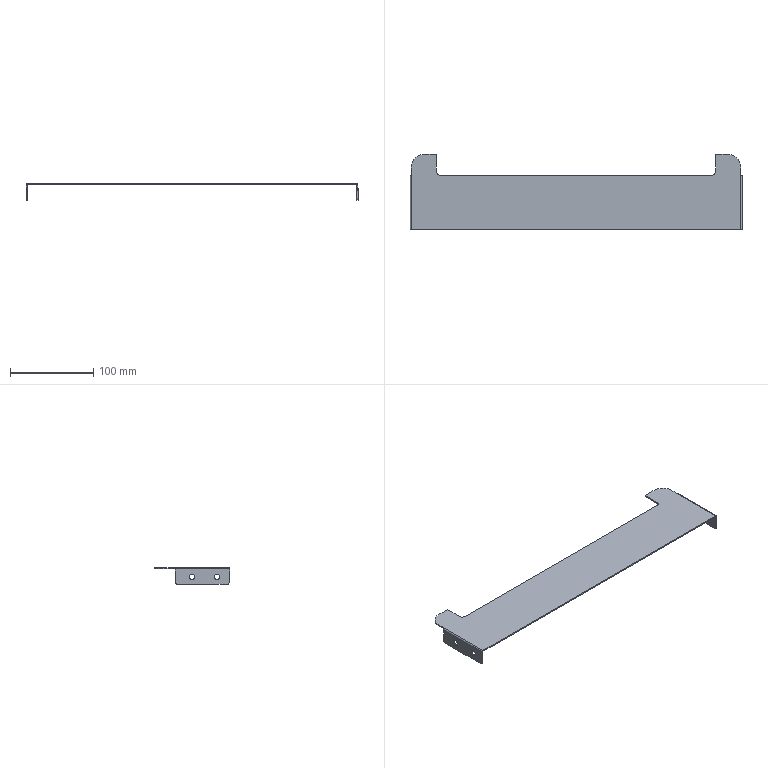Part | SolidWorks | features Fillet 3, EdgeFlange 1, FlatPattern 1, HoleWzd 1, ICE 1, SMBaseFlange 1, SheetMetal 1 | 1 solid | 42 faces | box 398 x 90 x 20 mm | volume 44260 mm3 | plane 24 | cylinder 18 | commonest cylinder face diameters 6.5 x8 6 x4 3 x2 10 x2 30 x2
STEP:
#1=CARTESIAN_POINT('',(199.,0.,-14.25));
#2=VERTEX_POINT('',#1);
#3=CARTESIAN_POINT('',(199.,0.,-7.75));
#4=VERTEX_POINT('',#3);
#5=CARTESIAN_POINT('',(199.,0.,-11.));
#6=DIRECTION('',(-1.,0.,0.));
#7=DIRECTION('',(0.,0.,1.));
#8=AXIS2_PLACEMENT_3D('',#5,#6,#7);
#9=CIRCLE('',#8,3.25);
#10=EDGE_CURVE('',#2,#4,#9,.T.);
#11=ORIENTED_EDGE('',*,*,#10,.F.);
#12=CARTESIAN_POINT('',(197.5,0.,-14.25));
#13=VERTEX_POINT('',#12);
#14=CARTESIAN_POINT('',(-199.,0.,-14.25));
#15=DIRECTION('',(-1.,0.,0.));
#16=VECTOR('',#15,1000.);
#17=LINE('',#14,#16);
#18=EDGE_CURVE('',#2,#13,#17,.T.);
#19=ORIENTED_EDGE('',*,*,#18,.T.);
#20=CARTESIAN_POINT('',(197.5,0.,-7.75));
#21=VERTEX_POINT('',#20);
#22=CARTESIAN_POINT('',(197.5,0.,-11.));
#23=DIRECTION('',(-1.,0.,0.));
#24=DIRECTION('',(0.,0.,1.));
#25=AXIS2_PLACEMENT_3D('',#22,#23,#24);
#26=CIRCLE('',#25,3.25);
#27=EDGE_CURVE('',#13,#21,#26,.T.);
#28=ORIENTED_EDGE('',*,*,#27,.T.);
#29=CARTESIAN_POINT('',(-199.,0.,-7.75));
#30=DIRECTION('',(-1.,0.,0.));
#31=VECTOR('',#30,1000.);
#32=LINE('',#29,#31);
#33=EDGE_CURVE('',#4,#21,#32,.T.);
#34=ORIENTED_EDGE('',*,*,#33,.F.);
#35=EDGE_LOOP('',(#11,#19,#28,#34));
#36=FACE_OUTER_BOUND('',#35,.T.);
#37=CARTESIAN_POINT('',(-199.,0.,-11.));
#38=DIRECTION('',(-1.,0.,0.));
#39=DIRECTION('',(0.,0.,1.));
#40=AXIS2_PLACEMENT_3D('',#37,#38,#39);
#41=CYLINDRICAL_SURFACE('',#40,3.25);
#42=ADVANCED_FACE('',(#36),#41,.F.);
#43=CARTESIAN_POINT('',(-197.5,0.,-14.25));
#44=VERTEX_POINT('',#43);
#45=CARTESIAN_POINT('',(-197.5,0.,-7.75));
#46=VERTEX_POINT('',#45);
#47=CARTESIAN_POINT('',(-197.5,0.,-11.));
#48=DIRECTION('',(-1.,0.,0.));
#49=DIRECTION('',(0.,0.,1.));
#50=AXIS2_PLACEMENT_3D('',#47,#48,#49);
#51=CIRCLE('',#50,3.25);
#52=EDGE_CURVE('',#44,#46,#51,.T.);
#53=ORIENTED_EDGE('',*,*,#52,.F.);
#54=CARTESIAN_POINT('',(-199.,0.,-14.25));
#55=VERTEX_POINT('',#54);
#56=CARTESIAN_POINT('',(-199.,0.,-14.25));
#57=DIRECTION('',(-1.,0.,0.));
#58=VECTOR('',#57,1000.);
#59=LINE('',#56,#58);
#60=EDGE_CURVE('',#44,#55,#59,.T.);
#61=ORIENTED_EDGE('',*,*,#60,.T.);
#62=CARTESIAN_POINT('',(-199.,0.,-7.75));
#63=VERTEX_POINT('',#62);
#64=CARTESIAN_POINT('',(-199.,0.,-11.));
#65=DIRECTION('',(-1.,0.,0.));
#66=DIRECTION('',(0.,0.,1.));
#67=AXIS2_PLACEMENT_3D('',#64,#65,#66);
#68=CIRCLE('',#67,3.25);
#69=EDGE_CURVE('',#55,#63,#68,.T.);
#70=ORIENTED_EDGE('',*,*,#69,.T.);
#71=CARTESIAN_POINT('',(-199.,0.,-7.75));
#72=DIRECTION('',(-1.,0.,0.));
#73=VECTOR('',#72,1000.);
#74=LINE('',#71,#73);
#75=EDGE_CURVE('',#46,#63,#74,.T.);
#76=ORIENTED_EDGE('',*,*,#75,.F.);
#77=EDGE_LOOP('',(#53,#61,#70,#76));
#78=FACE_OUTER_BOUND('',#77,.T.);
#79=CARTESIAN_POINT('',(-199.,0.,-11.));
#80=DIRECTION('',(-1.,0.,0.));
#81=DIRECTION('',(0.,0.,1.));
#82=AXIS2_PLACEMENT_3D('',#79,#80,#81);
#83=CYLINDRICAL_SURFACE('',#82,3.25);
#84=ADVANCED_FACE('',(#78),#83,.F.);
#85=CARTESIAN_POINT('',(-197.5,-30.,-14.25));
#86=VERTEX_POINT('',#85);
#87=CARTESIAN_POINT('',(-197.5,-30.,-7.75));
#88=VERTEX_POINT('',#87);
#89=CARTESIAN_POINT('',(-197.5,-30.,-11.));
#90=DIRECTION('',(-1.,0.,0.));
#91=DIRECTION('',(0.,0.,1.));
#92=AXIS2_PLACEMENT_3D('',#89,#90,#91);
#93=CIRCLE('',#92,3.25);
#94=EDGE_CURVE('',#86,#88,#93,.T.);
#95=ORIENTED_EDGE('',*,*,#94,.F.);
#96=CARTESIAN_POINT('',(-199.,-30.,-14.25));
#97=VERTEX_POINT('',#96);
#98=CARTESIAN_POINT('',(-199.,-30.,-14.25));
#99=DIRECTION('',(-1.,0.,0.));
#100=VECTOR('',#99,1000.);
#101=LINE('',#98,#100);
#102=EDGE_CURVE('',#86,#97,#101,.T.);
#103=ORIENTED_EDGE('',*,*,#102,.T.);
#104=CARTESIAN_POINT('',(-199.,-30.,-7.75));
#105=VERTEX_POINT('',#104);
#106=CARTESIAN_POINT('',(-199.,-30.,-11.));
#107=DIRECTION('',(-1.,0.,0.));
#108=DIRECTION('',(0.,0.,1.));
#109=AXIS2_PLACEMENT_3D('',#106,#107,#108);
#110=CIRCLE('',#109,3.25);
#111=EDGE_CURVE('',#97,#105,#110,.T.);
#112=ORIENTED_EDGE('',*,*,#111,.T.);
#113=CARTESIAN_POINT('',(-199.,-30.,-7.75));
#114=DIRECTION('',(-1.,0.,0.));
#115=VECTOR('',#114,1000.);
#116=LINE('',#113,#115);
#117=EDGE_CURVE('',#88,#105,#116,.T.);
#118=ORIENTED_EDGE('',*,*,#117,.F.);
#119=EDGE_LOOP('',(#95,#103,#112,#118));
#120=FACE_OUTER_BOUND('',#119,.T.);
#121=CARTESIAN_POINT('',(-199.,-30.,-11.));
#122=DIRECTION('',(-1.,0.,0.));
#123=DIRECTION('',(0.,0.,1.));
#124=AXIS2_PLACEMENT_3D('',#121,#122,#123);
#125=CYLINDRICAL_SURFACE('',#124,3.25);
#126=ADVANCED_FACE('',(#120),#125,.F.);
#127=CARTESIAN_POINT('',(199.,-30.,-14.25));
#128=VERTEX_POINT('',#127);
#129=CARTESIAN_POINT('',(199.,-30.,-7.75));
#130=VERTEX_POINT('',#129);
#131=CARTESIAN_POINT('',(199.,-30.,-11.));
#132=DIRECTION('',(-1.,0.,0.));
#133=DIRECTION('',(0.,0.,1.));
#134=AXIS2_PLACEMENT_3D('',#131,#132,#133);
#135=CIRCLE('',#134,3.25);
#136=EDGE_CURVE('',#128,#130,#135,.T.);
#137=ORIENTED_EDGE('',*,*,#136,.F.);
#138=CARTESIAN_POINT('',(197.5,-30.,-14.25));
#139=VERTEX_POINT('',#138);
#140=CARTESIAN_POINT('',(-199.,-30.,-14.25));
#141=DIRECTION('',(-1.,0.,0.));
#142=VECTOR('',#141,1000.);
#143=LINE('',#140,#142);
#144=EDGE_CURVE('',#128,#139,#143,.T.);
#145=ORIENTED_EDGE('',*,*,#144,.T.);
#146=CARTESIAN_POINT('',(197.5,-30.,-7.75));
#147=VERTEX_POINT('',#146);
#148=CARTESIAN_POINT('',(197.5,-30.,-11.));
#149=DIRECTION('',(-1.,0.,0.));
#150=DIRECTION('',(0.,0.,1.));
#151=AXIS2_PLACEMENT_3D('',#148,#149,#150);
#152=CIRCLE('',#151,3.25);
#153=EDGE_CURVE('',#139,#147,#152,.T.);
#154=ORIENTED_EDGE('',*,*,#153,.T.);
#155=CARTESIAN_POINT('',(-199.,-30.,-7.75));
#156=DIRECTION('',(-1.,0.,0.));
#157=VECTOR('',#156,1000.);
#158=LINE('',#155,#157);
#159=EDGE_CURVE('',#130,#147,#158,.T.);
#160=ORIENTED_EDGE('',*,*,#159,.F.);
#161=EDGE_LOOP('',(#137,#145,#154,#160));
#162=FACE_OUTER_BOUND('',#161,.T.);
#163=CARTESIAN_POINT('',(-199.,-30.,-11.));
#164=DIRECTION('',(-1.,0.,0.));
#165=DIRECTION('',(0.,0.,1.));
#166=AXIS2_PLACEMENT_3D('',#163,#164,#165);
#167=CYLINDRICAL_SURFACE('',#166,3.25);
#168=ADVANCED_FACE('',(#162),#167,.F.);
#169=CARTESIAN_POINT('',(-167.5,45.,-1.5));
#170=VERTEX_POINT('',#169);
#171=CARTESIAN_POINT('',(-167.5,45.,0.));
#172=VERTEX_POINT('',#171);
#173=CARTESIAN_POINT('',(-167.5,45.,-1.5));
#174=DIRECTION('',(0.,0.,1.));
#175=VECTOR('',#174,1000.);
#176=LINE('',#173,#175);
#177=EDGE_CURVE('',#170,#172,#176,.T.);
#178=ORIENTED_EDGE('',*,*,#177,.F.);
#179=CARTESIAN_POINT('',(-182.5,45.,-1.5));
#180=VERTEX_POINT('',#179);
#181=CARTESIAN_POINT('',(197.5,45.,-1.5));
#182=DIRECTION('',(-1.,0.,0.));
#183=VECTOR('',#182,1000.);
#184=LINE('',#181,#183);
#185=EDGE_CURVE('',#170,#180,#184,.T.);
#186=ORIENTED_EDGE('',*,*,#185,.T.);
#187=CARTESIAN_POINT('',(-182.5,45.,0.));
#188=VERTEX_POINT('',#187);
#189=CARTESIAN_POINT('',(-182.5,45.,-1.5));
#190=DIRECTION('',(0.,0.,1.));
#191=VECTOR('',#190,1000.);
#192=LINE('',#189,#191);
#193=EDGE_CURVE('',#180,#188,#192,.T.);
#194=ORIENTED_EDGE('',*,*,#193,.T.);
#195=CARTESIAN_POINT('',(197.5,45.,0.));
#196=DIRECTION('',(-1.,0.,0.));
#197=VECTOR('',#196,1000.);
#198=LINE('',#195,#197);
#199=EDGE_CURVE('',#172,#188,#198,.T.);
#200=ORIENTED_EDGE('',*,*,#199,.F.);
#201=EDGE_LOOP('',(#178,#186,#194,#200));
#202=FACE_OUTER_BOUND('',#201,.T.);
#203=CARTESIAN_POINT('',(197.5,45.,-1.5));
#204=DIRECTION('',(0.,1.,0.));
#205=DIRECTION('',(-1.,0.,0.));
#206=AXIS2_PLACEMENT_3D('',#203,#204,#205);
#207=PLANE('',#206);
#208=ADVANCED_FACE('',(#202),#207,.T.);
#209=CARTESIAN_POINT('',(197.5,20.,0.));
#210=VERTEX_POINT('',#209);
#211=CARTESIAN_POINT('',(197.5,30.,0.));
#212=VERTEX_POINT('',#211);
#213=CARTESIAN_POINT('',(197.5,-45.,0.));
#214=DIRECTION('',(0.,1.,0.));
#215=VECTOR('',#214,1000.);
#216=LINE('',#213,#215);
#217=EDGE_CURVE('',#210,#212,#216,.T.);
#218=ORIENTED_EDGE('',*,*,#217,.F.);
#219=CARTESIAN_POINT('',(197.5,20.,-1.5));
#220=VERTEX_POINT('',#219);
#221=CARTESIAN_POINT('',(197.5,20.,0.));
#222=DIRECTION('',(0.,0.,-1.));
#223=VECTOR('',#222,1000.);
#224=LINE('',#221,#223);
#225=EDGE_CURVE('',#210,#220,#224,.T.);
#226=ORIENTED_EDGE('',*,*,#225,.T.);
#227=CARTESIAN_POINT('',(197.5,30.,-1.5));
#228=VERTEX_POINT('',#227);
#229=CARTESIAN_POINT('',(197.5,-45.,-1.5));
#230=DIRECTION('',(0.,1.,0.));
#231=VECTOR('',#230,1000.);
#232=LINE('',#229,#231);
#233=EDGE_CURVE('',#220,#228,#232,.T.);
#234=ORIENTED_EDGE('',*,*,#233,.T.);
#235=CARTESIAN_POINT('',(197.5,30.,-1.5));
#236=DIRECTION('',(0.,0.,1.));
#237=VECTOR('',#236,1000.);
#238=LINE('',#235,#237);
#239=EDGE_CURVE('',#228,#212,#238,.T.);
#240=ORIENTED_EDGE('',*,*,#239,.T.);
#241=EDGE_LOOP('',(#218,#226,#234,#240));
#242=FACE_OUTER_BOUND('',#241,.T.);
#243=CARTESIAN_POINT('',(197.5,-45.,-1.5));
#244=DIRECTION('',(1.,0.,0.));
#245=DIRECTION('',(0.,0.,-1.));
#246=AXIS2_PLACEMENT_3D('',#243,#244,#245);
#247=PLANE('',#246);
#248=ADVANCED_FACE('',(#242),#247,.T.);
#249=CARTESIAN_POINT('',(-197.5,20.,0.));
#250=VERTEX_POINT('',#249);
#251=CARTESIAN_POINT('',(-197.5,20.,-1.5));
#252=VERTEX_POINT('',#251);
#253=CARTESIAN_POINT('',(-197.5,20.,0.));
#254=DIRECTION('',(0.,0.,-1.));
#255=VECTOR('',#254,1000.);
#256=LINE('',#253,#255);
#257=EDGE_CURVE('',#250,#252,#256,.T.);
#258=ORIENTED_EDGE('',*,*,#257,.F.);
#259=CARTESIAN_POINT('',(-197.5,30.,0.));
#260=VERTEX_POINT('',#259);
#261=CARTESIAN_POINT('',(-197.5,-45.,0.));
#262=DIRECTION('',(0.,-1.,0.));
#263=VECTOR('',#262,1000.);
#264=LINE('',#261,#263);
#265=EDGE_CURVE('',#260,#250,#264,.T.);
#266=ORIENTED_EDGE('',*,*,#265,.F.);
#267=CARTESIAN_POINT('',(-197.5,30.,-1.5));
#268=VERTEX_POINT('',#267);
#269=CARTESIAN_POINT('',(-197.5,30.,-1.5));
#270=DIRECTION('',(0.,0.,-1.));
#271=VECTOR('',#270,1000.);
#272=LINE('',#269,#271);
#273=EDGE_CURVE('',#260,#268,#272,.T.);
#274=ORIENTED_EDGE('',*,*,#273,.T.);
#275=CARTESIAN_POINT('',(-197.5,-45.,-1.5));
#276=DIRECTION('',(0.,-1.,0.));
#277=VECTOR('',#276,1000.);
#278=LINE('',#275,#277);
#279=EDGE_CURVE('',#268,#252,#278,.T.);
#280=ORIENTED_EDGE('',*,*,#279,.T.);
#281=EDGE_LOOP('',(#258,#266,#274,#280));
#282=FACE_OUTER_BOUND('',#281,.T.);
#283=CARTESIAN_POINT('',(-197.5,-45.,-1.5));
#284=DIRECTION('',(-1.,0.,0.));
#285=DIRECTION('',(0.,0.,1.));
#286=AXIS2_PLACEMENT_3D('',#283,#284,#285);
#287=PLANE('',#286);
#288=ADVANCED_FACE('',(#282),#287,.T.);
#289=CARTESIAN_POINT('',(167.5,45.,0.));
#290=VERTEX_POINT('',#289);
#291=CARTESIAN_POINT('',(167.5,45.,-1.5));
#292=VERTEX_POINT('',#291);
#293=CARTESIAN_POINT('',(167.5,45.,-1.5));
#294=DIRECTION('',(0.,0.,-1.));
#295=VECTOR('',#294,1000.);
#296=LINE('',#293,#295);
#297=EDGE_CURVE('',#290,#292,#296,.T.);
#298=ORIENTED_EDGE('',*,*,#297,.F.);
#299=CARTESIAN_POINT('',(182.5,45.,0.));
#300=VERTEX_POINT('',#299);
#301=CARTESIAN_POINT('',(197.5,45.,0.));
#302=DIRECTION('',(-1.,0.,0.));
#303=VECTOR('',#302,1000.);
#304=LINE('',#301,#303);
#305=EDGE_CURVE('',#300,#290,#304,.T.);
#306=ORIENTED_EDGE('',*,*,#305,.F.);
#307=CARTESIAN_POINT('',(182.5,45.,-1.5));
#308=VERTEX_POINT('',#307);
#309=CARTESIAN_POINT('',(182.5,45.,-1.5));
#310=DIRECTION('',(0.,0.,-1.));
#311=VECTOR('',#310,1000.);
#312=LINE('',#309,#311);
#313=EDGE_CURVE('',#300,#308,#312,.T.);
#314=ORIENTED_EDGE('',*,*,#313,.T.);
#315=CARTESIAN_POINT('',(197.5,45.,-1.5));
#316=DIRECTION('',(-1.,0.,0.));
#317=VECTOR('',#316,1000.);
#318=LINE('',#315,#317);
#319=EDGE_CURVE('',#308,#292,#318,.T.);
#320=ORIENTED_EDGE('',*,*,#319,.T.);
#321=EDGE_LOOP('',(#298,#306,#314,#320));
#322=FACE_OUTER_BOUND('',#321,.T.);
#323=CARTESIAN_POINT('',(197.5,45.,-1.5));
#324=DIRECTION('',(0.,1.,0.));
#325=DIRECTION('',(-1.,0.,0.));
#326=AXIS2_PLACEMENT_3D('',#323,#324,#325);
#327=PLANE('',#326);
#328=ADVANCED_FACE('',(#322),#327,.T.);
#329=CARTESIAN_POINT('',(-197.5,-45.,0.));
#330=VERTEX_POINT('',#329);
#331=CARTESIAN_POINT('',(197.5,-45.,0.));
#332=VERTEX_POINT('',#331);
#333=CARTESIAN_POINT('',(197.5,-45.,0.));
#334=DIRECTION('',(1.,0.,0.));
#335=VECTOR('',#334,1000.);
#336=LINE('',#333,#335);
#337=EDGE_CURVE('',#330,#332,#336,.T.);
#338=ORIENTED_EDGE('',*,*,#337,.F.);
#339=CARTESIAN_POINT('',(-197.5,-45.,-1.5));
#340=VERTEX_POINT('',#339);
#341=CARTESIAN_POINT('',(-197.5,-45.,-1.5));
#342=DIRECTION('',(0.,0.,1.));
#343=VECTOR('',#342,1000.);
#344=LINE('',#341,#343);
#345=EDGE_CURVE('',#340,#330,#344,.T.);
#346=ORIENTED_EDGE('',*,*,#345,.F.);
#347=CARTESIAN_POINT('',(197.5,-45.,-1.5));
#348=VERTEX_POINT('',#347);
#349=CARTESIAN_POINT('',(197.5,-45.,-1.5));
#350=DIRECTION('',(1.,0.,0.));
#351=VECTOR('',#350,1000.);
#352=LINE('',#349,#351);
#353=EDGE_CURVE('',#340,#348,#352,.T.);
#354=ORIENTED_EDGE('',*,*,#353,.T.);
#355=CARTESIAN_POINT('',(197.5,-45.,-1.5));
#356=DIRECTION('',(0.,0.,1.));
#357=VECTOR('',#356,1000.);
#358=LINE('',#355,#357);
#359=EDGE_CURVE('',#348,#332,#358,.T.);
#360=ORIENTED_EDGE('',*,*,#359,.T.);
#361=EDGE_LOOP('',(#338,#346,#354,#360));
#362=FACE_OUTER_BOUND('',#361,.T.);
#363=CARTESIAN_POINT('',(197.5,-45.,-1.5));
#364=DIRECTION('',(0.,-1.,0.));
#365=DIRECTION('',(1.,0.,0.));
#366=AXIS2_PLACEMENT_3D('',#363,#364,#365);
#367=PLANE('',#366);
#368=ADVANCED_FACE('',(#362),#367,.T.);
#369=ORIENTED_EDGE('',*,*,#185,.F.);
#370=CARTESIAN_POINT('',(-167.5,25.,-1.5));
#371=VERTEX_POINT('',#370);
#372=CARTESIAN_POINT('',(-167.5,0.,-1.5));
#373=DIRECTION('',(0.,-1.,0.));
#374=VECTOR('',#373,1000.);
#375=LINE('',#372,#374);
#376=EDGE_CURVE('',#170,#371,#375,.T.);
#377=ORIENTED_EDGE('',*,*,#376,.T.);
#378=CARTESIAN_POINT('',(-162.5,20.,-1.5));
#379=VERTEX_POINT('',#378);
#380=CARTESIAN_POINT('',(-162.5,25.,-1.5));
#381=DIRECTION('',(0.,0.,1.));
#382=DIRECTION('',(1.,0.,0.));
#383=AXIS2_PLACEMENT_3D('',#380,#381,#382);
#384=CIRCLE('',#383,5.);
#385=EDGE_CURVE('',#371,#379,#384,.T.);
#386=ORIENTED_EDGE('',*,*,#385,.T.);
#387=CARTESIAN_POINT('',(162.5,20.,-1.5));
#388=VERTEX_POINT('',#387);
#389=CARTESIAN_POINT('',(0.,20.,-1.5));
#390=DIRECTION('',(1.,0.,0.));
#391=VECTOR('',#390,1000.);
#392=LINE('',#389,#391);
#393=EDGE_CURVE('',#379,#388,#392,.T.);
#394=ORIENTED_EDGE('',*,*,#393,.T.);
#395=CARTESIAN_POINT('',(167.5,25.,-1.5));
#396=VERTEX_POINT('',#395);
#397=CARTESIAN_POINT('',(162.5,25.,-1.5));
#398=DIRECTION('',(0.,0.,1.));
#399=DIRECTION('',(1.,0.,0.));
#400=AXIS2_PLACEMENT_3D('',#397,#398,#399);
#401=CIRCLE('',#400,5.);
#402=EDGE_CURVE('',#388,#396,#401,.T.);
#403=ORIENTED_EDGE('',*,*,#402,.T.);
#404=CARTESIAN_POINT('',(167.5,0.,-1.5));
#405=DIRECTION('',(0.,1.,0.));
#406=VECTOR('',#405,1000.);
#407=LINE('',#404,#406);
#408=EDGE_CURVE('',#396,#292,#407,.T.);
#409=ORIENTED_EDGE('',*,*,#408,.T.);
#410=ORIENTED_EDGE('',*,*,#319,.F.);
#411=CARTESIAN_POINT('',(182.5,30.,-1.5));
#412=DIRECTION('',(0.,0.,-1.));
#413=DIRECTION('',(1.,0.,0.));
#414=AXIS2_PLACEMENT_3D('',#411,#412,#413);
#415=CIRCLE('',#414,15.);
#416=EDGE_CURVE('',#308,#228,#415,.T.);
#417=ORIENTED_EDGE('',*,*,#416,.T.);
#418=ORIENTED_EDGE('',*,*,#233,.F.);
#419=CARTESIAN_POINT('',(197.5,-45.,-1.5));
#420=DIRECTION('',(0.,1.,0.));
#421=VECTOR('',#420,1000.);
#422=LINE('',#419,#421);
#423=EDGE_CURVE('',#348,#220,#422,.T.);
#424=ORIENTED_EDGE('',*,*,#423,.F.);
#425=ORIENTED_EDGE('',*,*,#353,.F.);
#426=CARTESIAN_POINT('',(-197.5,-45.,-1.5));
#427=DIRECTION('',(0.,-1.,0.));
#428=VECTOR('',#427,1000.);
#429=LINE('',#426,#428);
#430=EDGE_CURVE('',#252,#340,#429,.T.);
#431=ORIENTED_EDGE('',*,*,#430,.F.);
#432=ORIENTED_EDGE('',*,*,#279,.F.);
#433=CARTESIAN_POINT('',(-182.5,30.,-1.5));
#434=DIRECTION('',(0.,0.,-1.));
#435=DIRECTION('',(1.,0.,0.));
#436=AXIS2_PLACEMENT_3D('',#433,#434,#435);
#437=CIRCLE('',#436,15.);
#438=EDGE_CURVE('',#268,#180,#437,.T.);
#439=ORIENTED_EDGE('',*,*,#438,.T.);
#440=EDGE_LOOP('',(#369,#377,#386,#394,#403,#409,#410,#417,#418,#424,#425,#431,#432,#439));
#441=FACE_OUTER_BOUND('',#440,.T.);
#442=CARTESIAN_POINT('',(0.,0.,-1.5));
#443=DIRECTION('',(0.,0.,1.));
#444=DIRECTION('',(1.,0.,0.));
#445=AXIS2_PLACEMENT_3D('',#442,#443,#444);
#446=PLANE('',#445);
#447=ADVANCED_FACE('',(#441),#446,.F.);
#448=CARTESIAN_POINT('',(-167.5,25.,0.));
#449=VERTEX_POINT('',#448);
#450=CARTESIAN_POINT('',(-167.5,0.,0.));
#451=DIRECTION('',(0.,-1.,0.));
#452=VECTOR('',#451,1000.);
#453=LINE('',#450,#452);
#454=EDGE_CURVE('',#172,#449,#453,.T.);
#455=ORIENTED_EDGE('',*,*,#454,.F.);
#456=ORIENTED_EDGE('',*,*,#199,.T.);
#457=CARTESIAN_POINT('',(-182.5,30.,0.));
#458=DIRECTION('',(0.,0.,1.));
#459=DIRECTION('',(1.,0.,0.));
#460=AXIS2_PLACEMENT_3D('',#457,#458,#459);
#461=CIRCLE('',#460,15.);
#462=EDGE_CURVE('',#188,#260,#461,.T.);
#463=ORIENTED_EDGE('',*,*,#462,.T.);
#464=ORIENTED_EDGE('',*,*,#265,.T.);
#465=CARTESIAN_POINT('',(-197.5,-45.,0.));
#466=DIRECTION('',(0.,-1.,0.));
#467=VECTOR('',#466,1000.);
#468=LINE('',#465,#467);
#469=EDGE_CURVE('',#250,#330,#468,.T.);
#470=ORIENTED_EDGE('',*,*,#469,.T.);
#471=ORIENTED_EDGE('',*,*,#337,.T.);
#472=CARTESIAN_POINT('',(197.5,-45.,0.));
#473=DIRECTION('',(0.,1.,0.));
#474=VECTOR('',#473,1000.);
#475=LINE('',#472,#474);
#476=EDGE_CURVE('',#332,#210,#475,.T.);
#477=ORIENTED_EDGE('',*,*,#476,.T.);
#478=ORIENTED_EDGE('',*,*,#217,.T.);
#479=CARTESIAN_POINT('',(182.5,30.,0.));
#480=DIRECTION('',(0.,0.,1.));
#481=DIRECTION('',(1.,0.,0.));
#482=AXIS2_PLACEMENT_3D('',#479,#480,#481);
#483=CIRCLE('',#482,15.);
#484=EDGE_CURVE('',#212,#300,#483,.T.);
#485=ORIENTED_EDGE('',*,*,#484,.T.);
#486=ORIENTED_EDGE('',*,*,#305,.T.);
#487=CARTESIAN_POINT('',(167.5,25.,0.));
#488=VERTEX_POINT('',#487);
#489=CARTESIAN_POINT('',(167.5,70.,0.));
#490=DIRECTION('',(0.,1.,0.));
#491=VECTOR('',#490,1000.);
#492=LINE('',#489,#491);
#493=EDGE_CURVE('',#488,#290,#492,.T.);
#494=ORIENTED_EDGE('',*,*,#493,.F.);
#495=CARTESIAN_POINT('',(162.5,20.,0.));
#496=VERTEX_POINT('',#495);
#497=CARTESIAN_POINT('',(162.5,25.,0.));
#498=DIRECTION('',(0.,0.,-1.));
#499=DIRECTION('',(1.,0.,0.));
#500=AXIS2_PLACEMENT_3D('',#497,#498,#499);
#501=CIRCLE('',#500,5.);
#502=EDGE_CURVE('',#488,#496,#501,.T.);
#503=ORIENTED_EDGE('',*,*,#502,.T.);
#504=CARTESIAN_POINT('',(-162.5,20.,0.));
#505=VERTEX_POINT('',#504);
#506=CARTESIAN_POINT('',(167.5,20.,0.));
#507=DIRECTION('',(1.,0.,0.));
#508=VECTOR('',#507,1000.);
#509=LINE('',#506,#508);
#510=EDGE_CURVE('',#505,#496,#509,.T.);
#511=ORIENTED_EDGE('',*,*,#510,.F.);
#512=CARTESIAN_POINT('',(-162.5,25.,0.));
#513=DIRECTION('',(0.,0.,-1.));
#514=DIRECTION('',(1.,0.,0.));
#515=AXIS2_PLACEMENT_3D('',#512,#513,#514);
#516=CIRCLE('',#515,5.);
#517=EDGE_CURVE('',#505,#449,#516,.T.);
#518=ORIENTED_EDGE('',*,*,#517,.T.);
#519=EDGE_LOOP('',(#455,#456,#463,#464,#470,#471,#477,#478,#485,#486,#494,#503,#511,#518));
#520=FACE_OUTER_BOUND('',#519,.T.);
#521=CARTESIAN_POINT('',(0.,0.,0.));
#522=DIRECTION('',(0.,0.,1.));
#523=DIRECTION('',(1.,0.,0.));
#524=AXIS2_PLACEMENT_3D('',#521,#522,#523);
#525=PLANE('',#524);
#526=ADVANCED_FACE('',(#520),#525,.T.);
#527=ORIENTED_EDGE('',*,*,#438,.F.);
#528=ORIENTED_EDGE('',*,*,#273,.F.);
#529=ORIENTED_EDGE('',*,*,#462,.F.);
#530=ORIENTED_EDGE('',*,*,#193,.F.);
#531=EDGE_LOOP('',(#527,#528,#529,#530));
#532=FACE_OUTER_BOUND('',#531,.T.);
#533=CARTESIAN_POINT('',(-182.5,30.,-1.5));
#534=DIRECTION('',(0.,0.,1.));
#535=DIRECTION('',(1.,0.,0.));
#536=AXIS2_PLACEMENT_3D('',#533,#534,#535);
#537=CYLINDRICAL_SURFACE('',#536,15.);
#538=ADVANCED_FACE('',(#532),#537,.T.);
#539=ORIENTED_EDGE('',*,*,#416,.F.);
#540=ORIENTED_EDGE('',*,*,#313,.F.);
#541=ORIENTED_EDGE('',*,*,#484,.F.);
#542=ORIENTED_EDGE('',*,*,#239,.F.);
#543=EDGE_LOOP('',(#539,#540,#541,#542));
#544=FACE_OUTER_BOUND('',#543,.T.);
#545=CARTESIAN_POINT('',(182.5,30.,-1.5));
#546=DIRECTION('',(0.,0.,1.));
#547=DIRECTION('',(1.,0.,0.));
#548=AXIS2_PLACEMENT_3D('',#545,#546,#547);
#549=CYLINDRICAL_SURFACE('',#548,15.);
#550=ADVANCED_FACE('',(#544),#549,.T.);
#551=CARTESIAN_POINT('',(-199.,20.,-1.5));
#552=VERTEX_POINT('',#551);
#553=CARTESIAN_POINT('',(-197.5,20.,-1.5));
#554=DIRECTION('',(0.,-1.,0.));
#555=DIRECTION('',(0.,0.,-1.));
#556=AXIS2_PLACEMENT_3D('',#553,#554,#555);
#557=CIRCLE('',#556,1.5);
#558=EDGE_CURVE('',#250,#552,#557,.T.);
#559=ORIENTED_EDGE('',*,*,#558,.F.);
#560=ORIENTED_EDGE('',*,*,#257,.T.);
#561=CARTESIAN_POINT('',(-199.,20.,-1.5));
#562=DIRECTION('',(1.,0.,0.));
#563=VECTOR('',#562,1000.);
#564=LINE('',#561,#563);
#565=EDGE_CURVE('',#552,#252,#564,.T.);
#566=ORIENTED_EDGE('',*,*,#565,.F.);
#567=EDGE_LOOP('',(#559,#560,#566));
#568=FACE_OUTER_BOUND('',#567,.T.);
#569=CARTESIAN_POINT('',(-197.5,20.,0.));
#570=DIRECTION('',(0.,1.,0.));
#571=DIRECTION('',(0.,0.,1.));
#572=AXIS2_PLACEMENT_3D('',#569,#570,#571);
#573=PLANE('',#572);
#574=ADVANCED_FACE('',(#568),#573,.T.);
#575=CARTESIAN_POINT('',(-199.,-45.,-1.5));
#576=VERTEX_POINT('',#575);
#577=CARTESIAN_POINT('',(-197.5,-45.,-1.5));
#578=DIRECTION('',(0.,-1.,0.));
#579=DIRECTION('',(0.,0.,-1.));
#580=AXIS2_PLACEMENT_3D('',#577,#578,#579);
#581=CIRCLE('',#580,1.5);
#582=EDGE_CURVE('',#330,#576,#581,.T.);
#583=ORIENTED_EDGE('',*,*,#582,.F.);
#584=ORIENTED_EDGE('',*,*,#469,.F.);
#585=ORIENTED_EDGE('',*,*,#558,.T.);
#586=CARTESIAN_POINT('',(-199.,-45.,-1.5));
#587=DIRECTION('',(0.,-1.,0.));
#588=VECTOR('',#587,1000.);
#589=LINE('',#586,#588);
#590=EDGE_CURVE('',#552,#576,#589,.T.);
#591=ORIENTED_EDGE('',*,*,#590,.T.);
#592=EDGE_LOOP('',(#583,#584,#585,#591));
#593=FACE_OUTER_BOUND('',#592,.T.);
#594=CARTESIAN_POINT('',(-197.5,-45.,-1.5));
#595=DIRECTION('',(0.,-1.,0.));
#596=DIRECTION('',(0.,0.,-1.));
#597=AXIS2_PLACEMENT_3D('',#594,#595,#596);
#598=CYLINDRICAL_SURFACE('',#597,1.5);
#599=ADVANCED_FACE('',(#593),#598,.T.);
#600=ORIENTED_EDGE('',*,*,#345,.T.);
#601=ORIENTED_EDGE('',*,*,#582,.T.);
#602=CARTESIAN_POINT('',(-199.,-45.,-1.5));
#603=DIRECTION('',(1.,0.,0.));
#604=VECTOR('',#603,1000.);
#605=LINE('',#602,#604);
#606=EDGE_CURVE('',#576,#340,#605,.T.);
#607=ORIENTED_EDGE('',*,*,#606,.T.);
#608=EDGE_LOOP('',(#600,#601,#607));
#609=FACE_OUTER_BOUND('',#608,.T.);
#610=CARTESIAN_POINT('',(-197.5,-45.,0.));
#611=DIRECTION('',(0.,1.,0.));
#612=DIRECTION('',(0.,0.,1.));
#613=AXIS2_PLACEMENT_3D('',#610,#611,#612);
#614=PLANE('',#613);
#615=ADVANCED_FACE('',(#609),#614,.F.);
#616=CARTESIAN_POINT('',(-197.5,20.,-17.));
#617=VERTEX_POINT('',#616);
#618=CARTESIAN_POINT('',(-197.5,20.,-1.5));
#619=DIRECTION('',(0.,0.,1.));
#620=VECTOR('',#619,1000.);
#621=LINE('',#618,#620);
#622=EDGE_CURVE('',#617,#252,#621,.T.);
#623=ORIENTED_EDGE('',*,*,#622,.F.);
#624=CARTESIAN_POINT('',(-199.,20.,-17.));
#625=VERTEX_POINT('',#624);
#626=CARTESIAN_POINT('',(-199.,20.,-17.));
#627=DIRECTION('',(-1.,0.,0.));
#628=VECTOR('',#627,1000.);
#629=LINE('',#626,#628);
#630=EDGE_CURVE('',#617,#625,#629,.T.);
#631=ORIENTED_EDGE('',*,*,#630,.T.);
#632=CARTESIAN_POINT('',(-199.,20.,-1.5));
#633=DIRECTION('',(0.,0.,1.));
#634=VECTOR('',#633,1000.);
#635=LINE('',#632,#634);
#636=EDGE_CURVE('',#625,#552,#635,.T.);
#637=ORIENTED_EDGE('',*,*,#636,.T.);
#638=ORIENTED_EDGE('',*,*,#565,.T.);
#639=EDGE_LOOP('',(#623,#631,#637,#638));
#640=FACE_OUTER_BOUND('',#639,.T.);
#641=CARTESIAN_POINT('',(-199.,20.,-1.5));
#642=DIRECTION('',(0.,1.,0.));
#643=DIRECTION('',(0.,0.,1.));
#644=AXIS2_PLACEMENT_3D('',#641,#642,#643);
#645=PLANE('',#644);
#646=ADVANCED_FACE('',(#640),#645,.T.);
#647=CARTESIAN_POINT('',(-197.5,-42.,-20.));
#648=VERTEX_POINT('',#647);
#649=CARTESIAN_POINT('',(-197.5,17.,-20.));
#650=VERTEX_POINT('',#649);
#651=CARTESIAN_POINT('',(-197.5,20.,-20.));
#652=DIRECTION('',(0.,1.,0.));
#653=VECTOR('',#652,1000.);
#654=LINE('',#651,#653);
#655=EDGE_CURVE('',#648,#650,#654,.T.);
#656=ORIENTED_EDGE('',*,*,#655,.F.);
#657=CARTESIAN_POINT('',(-199.,-42.,-20.));
#658=VERTEX_POINT('',#657);
#659=CARTESIAN_POINT('',(-199.,-42.,-20.));
#660=DIRECTION('',(-1.,0.,0.));
#661=VECTOR('',#660,1000.);
#662=LINE('',#659,#661);
#663=EDGE_CURVE('',#648,#658,#662,.T.);
#664=ORIENTED_EDGE('',*,*,#663,.T.);
#665=CARTESIAN_POINT('',(-199.,17.,-20.));
#666=VERTEX_POINT('',#665);
#667=CARTESIAN_POINT('',(-199.,20.,-20.));
#668=DIRECTION('',(0.,1.,0.));
#669=VECTOR('',#668,1000.);
#670=LINE('',#667,#669);
#671=EDGE_CURVE('',#658,#666,#670,.T.);
#672=ORIENTED_EDGE('',*,*,#671,.T.);
#673=CARTESIAN_POINT('',(-199.,17.,-20.));
#674=DIRECTION('',(1.,0.,0.));
#675=VECTOR('',#674,1000.);
#676=LINE('',#673,#675);
#677=EDGE_CURVE('',#666,#650,#676,.T.);
#678=ORIENTED_EDGE('',*,*,#677,.T.);
#679=EDGE_LOOP('',(#656,#664,#672,#678));
#680=FACE_OUTER_BOUND('',#679,.T.);
#681=CARTESIAN_POINT('',(-199.,20.,-20.));
#682=DIRECTION('',(0.,0.,-1.));
#683=DIRECTION('',(-1.,0.,0.));
#684=AXIS2_PLACEMENT_3D('',#681,#682,#683);
#685=PLANE('',#684);
#686=ADVANCED_FACE('',(#680),#685,.T.);
#687=CARTESIAN_POINT('',(-199.,-45.,-17.));
#688=VERTEX_POINT('',#687);
#689=CARTESIAN_POINT('',(-199.,-45.,-20.));
#690=DIRECTION('',(0.,0.,-1.));
#691=VECTOR('',#690,1000.);
#692=LINE('',#689,#691);
#693=EDGE_CURVE('',#576,#688,#692,.T.);
#694=ORIENTED_EDGE('',*,*,#693,.T.);
#695=CARTESIAN_POINT('',(-197.5,-45.,-17.));
#696=VERTEX_POINT('',#695);
#697=CARTESIAN_POINT('',(-199.,-45.,-17.));
#698=DIRECTION('',(1.,0.,0.));
#699=VECTOR('',#698,1000.);
#700=LINE('',#697,#699);
#701=EDGE_CURVE('',#688,#696,#700,.T.);
#702=ORIENTED_EDGE('',*,*,#701,.T.);
#703=CARTESIAN_POINT('',(-197.5,-45.,-20.));
#704=DIRECTION('',(0.,0.,-1.));
#705=VECTOR('',#704,1000.);
#706=LINE('',#703,#705);
#707=EDGE_CURVE('',#340,#696,#706,.T.);
#708=ORIENTED_EDGE('',*,*,#707,.F.);
#709=ORIENTED_EDGE('',*,*,#606,.F.);
#710=EDGE_LOOP('',(#694,#702,#708,#709));
#711=FACE_OUTER_BOUND('',#710,.T.);
#712=CARTESIAN_POINT('',(-199.,-45.,-20.));
#713=DIRECTION('',(0.,-1.,0.));
#714=DIRECTION('',(0.,0.,-1.));
#715=AXIS2_PLACEMENT_3D('',#712,#713,#714);
#716=PLANE('',#715);
#717=ADVANCED_FACE('',(#711),#716,.T.);
#718=CARTESIAN_POINT('',(-199.,0.,-11.));
#719=DIRECTION('',(-1.,0.,0.));
#720=DIRECTION('',(0.,0.,1.));
#721=AXIS2_PLACEMENT_3D('',#718,#719,#720);
#722=CIRCLE('',#721,3.25);
#723=EDGE_CURVE('',#63,#55,#722,.T.);
#724=ORIENTED_EDGE('',*,*,#723,.F.);
#725=ORIENTED_EDGE('',*,*,#69,.F.);
#726=EDGE_LOOP('',(#724,#725));
#727=FACE_BOUND('',#726,.T.);
#728=CARTESIAN_POINT('',(-199.,-30.,-11.));
#729=DIRECTION('',(-1.,0.,0.));
#730=DIRECTION('',(0.,0.,1.));
#731=AXIS2_PLACEMENT_3D('',#728,#729,#730);
#732=CIRCLE('',#731,3.25);
#733=EDGE_CURVE('',#105,#97,#732,.T.);
#734=ORIENTED_EDGE('',*,*,#733,.F.);
#735=ORIENTED_EDGE('',*,*,#111,.F.);
#736=EDGE_LOOP('',(#734,#735));
#737=FACE_BOUND('',#736,.T.);
#738=ORIENTED_EDGE('',*,*,#671,.F.);
#739=CARTESIAN_POINT('',(-199.,-42.,-17.));
#740=DIRECTION('',(-1.,0.,0.));
#741=DIRECTION('',(0.,0.,1.));
#742=AXIS2_PLACEMENT_3D('',#739,#740,#741);
#743=CIRCLE('',#742,3.);
#744=EDGE_CURVE('',#658,#688,#743,.T.);
#745=ORIENTED_EDGE('',*,*,#744,.T.);
#746=ORIENTED_EDGE('',*,*,#693,.F.);
#747=ORIENTED_EDGE('',*,*,#590,.F.);
#748=ORIENTED_EDGE('',*,*,#636,.F.);
#749=CARTESIAN_POINT('',(-199.,17.,-17.));
#750=DIRECTION('',(-1.,0.,0.));
#751=DIRECTION('',(0.,0.,1.));
#752=AXIS2_PLACEMENT_3D('',#749,#750,#751);
#753=CIRCLE('',#752,3.);
#754=EDGE_CURVE('',#625,#666,#753,.T.);
#755=ORIENTED_EDGE('',*,*,#754,.T.);
#756=EDGE_LOOP('',(#738,#745,#746,#747,#748,#755));
#757=FACE_OUTER_BOUND('',#756,.T.);
#758=CARTESIAN_POINT('',(-199.,0.,0.));
#759=DIRECTION('',(-1.,0.,0.));
#760=DIRECTION('',(0.,0.,1.));
#761=AXIS2_PLACEMENT_3D('',#758,#759,#760);
#762=PLANE('',#761);
#763=ADVANCED_FACE('',(#727,#737,#757),#762,.T.);
#764=CARTESIAN_POINT('',(-197.5,0.,-11.));
#765=DIRECTION('',(-1.,0.,0.));
#766=DIRECTION('',(0.,0.,1.));
#767=AXIS2_PLACEMENT_3D('',#764,#765,#766);
#768=CIRCLE('',#767,3.25);
#769=EDGE_CURVE('',#46,#44,#768,.T.);
#770=ORIENTED_EDGE('',*,*,#769,.T.);
#771=ORIENTED_EDGE('',*,*,#52,.T.);
#772=EDGE_LOOP('',(#770,#771));
#773=FACE_BOUND('',#772,.T.);
#774=CARTESIAN_POINT('',(-197.5,-30.,-11.));
#775=DIRECTION('',(-1.,0.,0.));
#776=DIRECTION('',(0.,0.,1.));
#777=AXIS2_PLACEMENT_3D('',#774,#775,#776);
#778=CIRCLE('',#777,3.25);
#779=EDGE_CURVE('',#88,#86,#778,.T.);
#780=ORIENTED_EDGE('',*,*,#779,.T.);
#781=ORIENTED_EDGE('',*,*,#94,.T.);
#782=EDGE_LOOP('',(#780,#781));
#783=FACE_BOUND('',#782,.T.);
#784=ORIENTED_EDGE('',*,*,#707,.T.);
#785=CARTESIAN_POINT('',(-197.5,-42.,-17.));
#786=DIRECTION('',(1.,0.,0.));
#787=DIRECTION('',(0.,0.,1.));
#788=AXIS2_PLACEMENT_3D('',#785,#786,#787);
#789=CIRCLE('',#788,3.);
#790=EDGE_CURVE('',#696,#648,#789,.T.);
#791=ORIENTED_EDGE('',*,*,#790,.T.);
#792=ORIENTED_EDGE('',*,*,#655,.T.);
#793=CARTESIAN_POINT('',(-197.5,17.,-17.));
#794=DIRECTION('',(1.,0.,0.));
#795=DIRECTION('',(0.,0.,1.));
#796=AXIS2_PLACEMENT_3D('',#793,#794,#795);
#797=CIRCLE('',#796,3.);
#798=EDGE_CURVE('',#650,#617,#797,.T.);
#799=ORIENTED_EDGE('',*,*,#798,.T.);
#800=ORIENTED_EDGE('',*,*,#622,.T.);
#801=ORIENTED_EDGE('',*,*,#430,.T.);
#802=EDGE_LOOP('',(#784,#791,#792,#799,#800,#801));
#803=FACE_OUTER_BOUND('',#802,.T.);
#804=CARTESIAN_POINT('',(-197.5,0.,0.));
#805=DIRECTION('',(-1.,0.,0.));
#806=DIRECTION('',(0.,0.,1.));
#807=AXIS2_PLACEMENT_3D('',#804,#805,#806);
#808=PLANE('',#807);
#809=ADVANCED_FACE('',(#773,#783,#803),#808,.F.);
#810=CARTESIAN_POINT('',(199.,-45.,-1.5));
#811=VERTEX_POINT('',#810);
#812=CARTESIAN_POINT('',(197.5,-45.,-1.5));
#813=DIRECTION('',(0.,1.,0.));
#814=DIRECTION('',(0.,0.,1.));
#815=AXIS2_PLACEMENT_3D('',#812,#813,#814);
#816=CIRCLE('',#815,1.5);
#817=EDGE_CURVE('',#332,#811,#816,.T.);
#818=ORIENTED_EDGE('',*,*,#817,.F.);
#819=ORIENTED_EDGE('',*,*,#359,.F.);
#820=CARTESIAN_POINT('',(199.,-45.,-1.5));
#821=DIRECTION('',(-1.,0.,0.));
#822=VECTOR('',#821,1000.);
#823=LINE('',#820,#822);
#824=EDGE_CURVE('',#811,#348,#823,.T.);
#825=ORIENTED_EDGE('',*,*,#824,.F.);
#826=EDGE_LOOP('',(#818,#819,#825));
#827=FACE_OUTER_BOUND('',#826,.T.);
#828=CARTESIAN_POINT('',(197.5,-45.,0.));
#829=DIRECTION('',(0.,-1.,0.));
#830=DIRECTION('',(0.,0.,-1.));
#831=AXIS2_PLACEMENT_3D('',#828,#829,#830);
#832=PLANE('',#831);
#833=ADVANCED_FACE('',(#827),#832,.T.);
#834=CARTESIAN_POINT('',(199.,20.,-1.5));
#835=VERTEX_POINT('',#834);
#836=CARTESIAN_POINT('',(197.5,20.,-1.5));
#837=DIRECTION('',(0.,1.,0.));
#838=DIRECTION('',(0.,0.,1.));
#839=AXIS2_PLACEMENT_3D('',#836,#837,#838);
#840=CIRCLE('',#839,1.5);
#841=EDGE_CURVE('',#210,#835,#840,.T.);
#842=ORIENTED_EDGE('',*,*,#841,.F.);
#843=ORIENTED_EDGE('',*,*,#476,.F.);
#844=ORIENTED_EDGE('',*,*,#817,.T.);
#845=CARTESIAN_POINT('',(199.,20.,-1.5));
#846=DIRECTION('',(0.,1.,0.));
#847=VECTOR('',#846,1000.);
#848=LINE('',#845,#847);
#849=EDGE_CURVE('',#811,#835,#848,.T.);
#850=ORIENTED_EDGE('',*,*,#849,.T.);
#851=EDGE_LOOP('',(#842,#843,#844,#850));
#852=FACE_OUTER_BOUND('',#851,.T.);
#853=CARTESIAN_POINT('',(197.5,20.,-1.5));
#854=DIRECTION('',(0.,1.,0.));
#855=DIRECTION('',(0.,0.,1.));
#856=AXIS2_PLACEMENT_3D('',#853,#854,#855);
#857=CYLINDRICAL_SURFACE('',#856,1.5);
#858=ADVANCED_FACE('',(#852),#857,.T.);
#859=ORIENTED_EDGE('',*,*,#225,.F.);
#860=ORIENTED_EDGE('',*,*,#841,.T.);
#861=CARTESIAN_POINT('',(199.,20.,-1.5));
#862=DIRECTION('',(-1.,0.,0.));
#863=VECTOR('',#862,1000.);
#864=LINE('',#861,#863);
#865=EDGE_CURVE('',#835,#220,#864,.T.);
#866=ORIENTED_EDGE('',*,*,#865,.T.);
#867=EDGE_LOOP('',(#859,#860,#866));
#868=FACE_OUTER_BOUND('',#867,.T.);
#869=CARTESIAN_POINT('',(197.5,20.,0.));
#870=DIRECTION('',(0.,-1.,0.));
#871=DIRECTION('',(0.,0.,-1.));
#872=AXIS2_PLACEMENT_3D('',#869,#870,#871);
#873=PLANE('',#872);
#874=ADVANCED_FACE('',(#868),#873,.F.);
#875=CARTESIAN_POINT('',(199.,20.,-17.));
#876=VERTEX_POINT('',#875);
#877=CARTESIAN_POINT('',(199.,20.,-1.5));
#878=DIRECTION('',(0.,0.,-1.));
#879=VECTOR('',#878,1000.);
#880=LINE('',#877,#879);
#881=EDGE_CURVE('',#835,#876,#880,.T.);
#882=ORIENTED_EDGE('',*,*,#881,.T.);
#883=CARTESIAN_POINT('',(197.5,20.,-17.));
#884=VERTEX_POINT('',#883);
#885=CARTESIAN_POINT('',(199.,20.,-17.));
#886=DIRECTION('',(-1.,0.,0.));
#887=VECTOR('',#886,1000.);
#888=LINE('',#885,#887);
#889=EDGE_CURVE('',#876,#884,#888,.T.);
#890=ORIENTED_EDGE('',*,*,#889,.T.);
#891=CARTESIAN_POINT('',(197.5,20.,-1.5));
#892=DIRECTION('',(0.,0.,-1.));
#893=VECTOR('',#892,1000.);
#894=LINE('',#891,#893);
#895=EDGE_CURVE('',#220,#884,#894,.T.);
#896=ORIENTED_EDGE('',*,*,#895,.F.);
#897=ORIENTED_EDGE('',*,*,#865,.F.);
#898=EDGE_LOOP('',(#882,#890,#896,#897));
#899=FACE_OUTER_BOUND('',#898,.T.);
#900=CARTESIAN_POINT('',(199.,20.,-1.5));
#901=DIRECTION('',(0.,1.,0.));
#902=DIRECTION('',(0.,0.,1.));
#903=AXIS2_PLACEMENT_3D('',#900,#901,#902);
#904=PLANE('',#903);
#905=ADVANCED_FACE('',(#899),#904,.T.);
#906=CARTESIAN_POINT('',(197.5,-45.,-17.));
#907=VERTEX_POINT('',#906);
#908=CARTESIAN_POINT('',(197.5,-45.,-20.));
#909=DIRECTION('',(0.,0.,1.));
#910=VECTOR('',#909,1000.);
#911=LINE('',#908,#910);
#912=EDGE_CURVE('',#907,#348,#911,.T.);
#913=ORIENTED_EDGE('',*,*,#912,.F.);
#914=CARTESIAN_POINT('',(199.,-45.,-17.));
#915=VERTEX_POINT('',#914);
#916=CARTESIAN_POINT('',(199.,-45.,-17.));
#917=DIRECTION('',(1.,0.,0.));
#918=VECTOR('',#917,1000.);
#919=LINE('',#916,#918);
#920=EDGE_CURVE('',#907,#915,#919,.T.);
#921=ORIENTED_EDGE('',*,*,#920,.T.);
#922=CARTESIAN_POINT('',(199.,-45.,-20.));
#923=DIRECTION('',(0.,0.,1.));
#924=VECTOR('',#923,1000.);
#925=LINE('',#922,#924);
#926=EDGE_CURVE('',#915,#811,#925,.T.);
#927=ORIENTED_EDGE('',*,*,#926,.T.);
#928=ORIENTED_EDGE('',*,*,#824,.T.);
#929=EDGE_LOOP('',(#913,#921,#927,#928));
#930=FACE_OUTER_BOUND('',#929,.T.);
#931=CARTESIAN_POINT('',(199.,-45.,-20.));
#932=DIRECTION('',(0.,-1.,0.));
#933=DIRECTION('',(0.,0.,-1.));
#934=AXIS2_PLACEMENT_3D('',#931,#932,#933);
#935=PLANE('',#934);
#936=ADVANCED_FACE('',(#930),#935,.T.);
#937=CARTESIAN_POINT('',(199.,17.,-20.));
#938=VERTEX_POINT('',#937);
#939=CARTESIAN_POINT('',(199.,-42.,-20.));
#940=VERTEX_POINT('',#939);
#941=CARTESIAN_POINT('',(199.,20.,-20.));
#942=DIRECTION('',(0.,-1.,0.));
#943=VECTOR('',#942,1000.);
#944=LINE('',#941,#943);
#945=EDGE_CURVE('',#938,#940,#944,.T.);
#946=ORIENTED_EDGE('',*,*,#945,.T.);
#947=CARTESIAN_POINT('',(197.5,-42.,-20.));
#948=VERTEX_POINT('',#947);
#949=CARTESIAN_POINT('',(199.,-42.,-20.));
#950=DIRECTION('',(-1.,0.,0.));
#951=VECTOR('',#950,1000.);
#952=LINE('',#949,#951);
#953=EDGE_CURVE('',#940,#948,#952,.T.);
#954=ORIENTED_EDGE('',*,*,#953,.T.);
#955=CARTESIAN_POINT('',(197.5,17.,-20.));
#956=VERTEX_POINT('',#955);
#957=CARTESIAN_POINT('',(197.5,20.,-20.));
#958=DIRECTION('',(0.,-1.,0.));
#959=VECTOR('',#958,1000.);
#960=LINE('',#957,#959);
#961=EDGE_CURVE('',#956,#948,#960,.T.);
#962=ORIENTED_EDGE('',*,*,#961,.F.);
#963=CARTESIAN_POINT('',(199.,17.,-20.));
#964=DIRECTION('',(1.,0.,0.));
#965=VECTOR('',#964,1000.);
#966=LINE('',#963,#965);
#967=EDGE_CURVE('',#956,#938,#966,.T.);
#968=ORIENTED_EDGE('',*,*,#967,.T.);
#969=EDGE_LOOP('',(#946,#954,#962,#968));
#970=FACE_OUTER_BOUND('',#969,.T.);
#971=CARTESIAN_POINT('',(199.,20.,-20.));
#972=DIRECTION('',(0.,0.,-1.));
#973=DIRECTION('',(-1.,0.,0.));
#974=AXIS2_PLACEMENT_3D('',#971,#972,#973);
#975=PLANE('',#974);
#976=ADVANCED_FACE('',(#970),#975,.T.);
#977=CARTESIAN_POINT('',(199.,0.,-11.));
#978=DIRECTION('',(-1.,0.,0.));
#979=DIRECTION('',(0.,0.,1.));
#980=AXIS2_PLACEMENT_3D('',#977,#978,#979);
#981=CIRCLE('',#980,3.25);
#982=EDGE_CURVE('',#4,#2,#981,.T.);
#983=ORIENTED_EDGE('',*,*,#982,.T.);
#984=ORIENTED_EDGE('',*,*,#10,.T.);
#985=EDGE_LOOP('',(#983,#984));
#986=FACE_BOUND('',#985,.T.);
#987=CARTESIAN_POINT('',(199.,-30.,-11.));
#988=DIRECTION('',(-1.,0.,0.));
#989=DIRECTION('',(0.,0.,1.));
#990=AXIS2_PLACEMENT_3D('',#987,#988,#989);
#991=CIRCLE('',#990,3.25);
#992=EDGE_CURVE('',#130,#128,#991,.T.);
#993=ORIENTED_EDGE('',*,*,#992,.T.);
#994=ORIENTED_EDGE('',*,*,#136,.T.);
#995=EDGE_LOOP('',(#993,#994));
#996=FACE_BOUND('',#995,.T.);
#997=ORIENTED_EDGE('',*,*,#926,.F.);
#998=CARTESIAN_POINT('',(199.,-42.,-17.));
#999=DIRECTION('',(1.,0.,0.));
#1000=DIRECTION('',(0.,0.,1.));
#1001=AXIS2_PLACEMENT_3D('',#998,#999,#1000);
#1002=CIRCLE('',#1001,3.);
#1003=EDGE_CURVE('',#915,#940,#1002,.T.);
#1004=ORIENTED_EDGE('',*,*,#1003,.T.);
#1005=ORIENTED_EDGE('',*,*,#945,.F.);
#1006=CARTESIAN_POINT('',(199.,17.,-17.));
#1007=DIRECTION('',(1.,0.,0.));
#1008=DIRECTION('',(0.,0.,1.));
#1009=AXIS2_PLACEMENT_3D('',#1006,#1007,#1008);
#1010=CIRCLE('',#1009,3.);
#1011=EDGE_CURVE('',#938,#876,#1010,.T.);
#1012=ORIENTED_EDGE('',*,*,#1011,.T.);
#1013=ORIENTED_EDGE('',*,*,#881,.F.);
#1014=ORIENTED_EDGE('',*,*,#849,.F.);
#1015=EDGE_LOOP('',(#997,#1004,#1005,#1012,#1013,#1014));
#1016=FACE_OUTER_BOUND('',#1015,.T.);
#1017=CARTESIAN_POINT('',(199.,0.,0.));
#1018=DIRECTION('',(-1.,0.,0.));
#1019=DIRECTION('',(0.,0.,1.));
#1020=AXIS2_PLACEMENT_3D('',#1017,#1018,#1019);
#1021=PLANE('',#1020);
#1022=ADVANCED_FACE('',(#986,#996,#1016),#1021,.F.);
#1023=CARTESIAN_POINT('',(197.5,0.,-11.));
#1024=DIRECTION('',(-1.,0.,0.));
#1025=DIRECTION('',(0.,0.,1.));
#1026=AXIS2_PLACEMENT_3D('',#1023,#1024,#1025);
#1027=CIRCLE('',#1026,3.25);
#1028=EDGE_CURVE('',#21,#13,#1027,.T.);
#1029=ORIENTED_EDGE('',*,*,#1028,.F.);
#1030=ORIENTED_EDGE('',*,*,#27,.F.);
#1031=EDGE_LOOP('',(#1029,#1030));
#1032=FACE_BOUND('',#1031,.T.);
#1033=CARTESIAN_POINT('',(197.5,-30.,-11.));
#1034=DIRECTION('',(-1.,0.,0.));
#1035=DIRECTION('',(0.,0.,1.));
#1036=AXIS2_PLACEMENT_3D('',#1033,#1034,#1035);
#1037=CIRCLE('',#1036,3.25);
#1038=EDGE_CURVE('',#147,#139,#1037,.T.);
#1039=ORIENTED_EDGE('',*,*,#1038,.F.);
#1040=ORIENTED_EDGE('',*,*,#153,.F.);
#1041=EDGE_LOOP('',(#1039,#1040));
#1042=FACE_BOUND('',#1041,.T.);
#1043=ORIENTED_EDGE('',*,*,#961,.T.);
#1044=CARTESIAN_POINT('',(197.5,-42.,-17.));
#1045=DIRECTION('',(-1.,0.,0.));
#1046=DIRECTION('',(0.,0.,1.));
#1047=AXIS2_PLACEMENT_3D('',#1044,#1045,#1046);
#1048=CIRCLE('',#1047,3.);
#1049=EDGE_CURVE('',#948,#907,#1048,.T.);
#1050=ORIENTED_EDGE('',*,*,#1049,.T.);
#1051=ORIENTED_EDGE('',*,*,#912,.T.);
#1052=ORIENTED_EDGE('',*,*,#423,.T.);
#1053=ORIENTED_EDGE('',*,*,#895,.T.);
#1054=CARTESIAN_POINT('',(197.5,17.,-17.));
#1055=DIRECTION('',(-1.,0.,0.));
#1056=DIRECTION('',(0.,0.,1.));
#1057=AXIS2_PLACEMENT_3D('',#1054,#1055,#1056);
#1058=CIRCLE('',#1057,3.);
#1059=EDGE_CURVE('',#884,#956,#1058,.T.);
#1060=ORIENTED_EDGE('',*,*,#1059,.T.);
#1061=EDGE_LOOP('',(#1043,#1050,#1051,#1052,#1053,#1060));
#1062=FACE_OUTER_BOUND('',#1061,.T.);
#1063=CARTESIAN_POINT('',(197.5,0.,0.));
#1064=DIRECTION('',(-1.,0.,0.));
#1065=DIRECTION('',(0.,0.,1.));
#1066=AXIS2_PLACEMENT_3D('',#1063,#1064,#1065);
#1067=PLANE('',#1066);
#1068=ADVANCED_FACE('',(#1032,#1042,#1062),#1067,.T.);
#1069=ORIENTED_EDGE('',*,*,#144,.F.);
#1070=ORIENTED_EDGE('',*,*,#992,.F.);
#1071=ORIENTED_EDGE('',*,*,#159,.T.);
#1072=ORIENTED_EDGE('',*,*,#1038,.T.);
#1073=EDGE_LOOP('',(#1069,#1070,#1071,#1072));
#1074=FACE_OUTER_BOUND('',#1073,.T.);
#1075=CARTESIAN_POINT('',(-199.,-30.,-11.));
#1076=DIRECTION('',(-1.,0.,0.));
#1077=DIRECTION('',(0.,0.,1.));
#1078=AXIS2_PLACEMENT_3D('',#1075,#1076,#1077);
#1079=CYLINDRICAL_SURFACE('',#1078,3.25);
#1080=ADVANCED_FACE('',(#1074),#1079,.F.);
#1081=ORIENTED_EDGE('',*,*,#102,.F.);
#1082=ORIENTED_EDGE('',*,*,#779,.F.);
#1083=ORIENTED_EDGE('',*,*,#117,.T.);
#1084=ORIENTED_EDGE('',*,*,#733,.T.);
#1085=EDGE_LOOP('',(#1081,#1082,#1083,#1084));
#1086=FACE_OUTER_BOUND('',#1085,.T.);
#1087=CARTESIAN_POINT('',(-199.,-30.,-11.));
#1088=DIRECTION('',(-1.,0.,0.));
#1089=DIRECTION('',(0.,0.,1.));
#1090=AXIS2_PLACEMENT_3D('',#1087,#1088,#1089);
#1091=CYLINDRICAL_SURFACE('',#1090,3.25);
#1092=ADVANCED_FACE('',(#1086),#1091,.F.);
#1093=ORIENTED_EDGE('',*,*,#60,.F.);
#1094=ORIENTED_EDGE('',*,*,#769,.F.);
#1095=ORIENTED_EDGE('',*,*,#75,.T.);
#1096=ORIENTED_EDGE('',*,*,#723,.T.);
#1097=EDGE_LOOP('',(#1093,#1094,#1095,#1096));
#1098=FACE_OUTER_BOUND('',#1097,.T.);
#1099=CARTESIAN_POINT('',(-199.,0.,-11.));
#1100=DIRECTION('',(-1.,0.,0.));
#1101=DIRECTION('',(0.,0.,1.));
#1102=AXIS2_PLACEMENT_3D('',#1099,#1100,#1101);
#1103=CYLINDRICAL_SURFACE('',#1102,3.25);
#1104=ADVANCED_FACE('',(#1098),#1103,.F.);
#1105=ORIENTED_EDGE('',*,*,#18,.F.);
#1106=ORIENTED_EDGE('',*,*,#982,.F.);
#1107=ORIENTED_EDGE('',*,*,#33,.T.);
#1108=ORIENTED_EDGE('',*,*,#1028,.T.);
#1109=EDGE_LOOP('',(#1105,#1106,#1107,#1108));
#1110=FACE_OUTER_BOUND('',#1109,.T.);
#1111=CARTESIAN_POINT('',(-199.,0.,-11.));
#1112=DIRECTION('',(-1.,0.,0.));
#1113=DIRECTION('',(0.,0.,1.));
#1114=AXIS2_PLACEMENT_3D('',#1111,#1112,#1113);
#1115=CYLINDRICAL_SURFACE('',#1114,3.25);
#1116=ADVANCED_FACE('',(#1110),#1115,.F.);
#1117=ORIENTED_EDGE('',*,*,#510,.T.);
#1118=CARTESIAN_POINT('',(162.5,20.,-1.5));
#1119=DIRECTION('',(0.,0.,-1.));
#1120=VECTOR('',#1119,1000.);
#1121=LINE('',#1118,#1120);
#1122=EDGE_CURVE('',#496,#388,#1121,.T.);
#1123=ORIENTED_EDGE('',*,*,#1122,.T.);
#1124=ORIENTED_EDGE('',*,*,#393,.F.);
#1125=CARTESIAN_POINT('',(-162.5,20.,0.));
#1126=DIRECTION('',(0.,0.,1.));
#1127=VECTOR('',#1126,1000.);
#1128=LINE('',#1125,#1127);
#1129=EDGE_CURVE('',#379,#505,#1128,.T.);
#1130=ORIENTED_EDGE('',*,*,#1129,.T.);
#1131=EDGE_LOOP('',(#1117,#1123,#1124,#1130));
#1132=FACE_OUTER_BOUND('',#1131,.T.);
#1133=CARTESIAN_POINT('',(167.5,20.,-10.));
#1134=DIRECTION('',(0.,-1.,0.));
#1135=DIRECTION('',(0.,0.,-1.));
#1136=AXIS2_PLACEMENT_3D('',#1133,#1134,#1135);
#1137=PLANE('',#1136);
#1138=ADVANCED_FACE('',(#1132),#1137,.F.);
#1139=ORIENTED_EDGE('',*,*,#454,.T.);
#1140=CARTESIAN_POINT('',(-167.5,25.,-1.5));
#1141=DIRECTION('',(0.,0.,-1.));
#1142=VECTOR('',#1141,1000.);
#1143=LINE('',#1140,#1142);
#1144=EDGE_CURVE('',#449,#371,#1143,.T.);
#1145=ORIENTED_EDGE('',*,*,#1144,.T.);
#1146=ORIENTED_EDGE('',*,*,#376,.F.);
#1147=ORIENTED_EDGE('',*,*,#177,.T.);
#1148=EDGE_LOOP('',(#1139,#1145,#1146,#1147));
#1149=FACE_OUTER_BOUND('',#1148,.T.);
#1150=CARTESIAN_POINT('',(-167.5,70.,-10.));
#1151=DIRECTION('',(-1.,0.,0.));
#1152=DIRECTION('',(0.,0.,1.));
#1153=AXIS2_PLACEMENT_3D('',#1150,#1151,#1152);
#1154=PLANE('',#1153);
#1155=ADVANCED_FACE('',(#1149),#1154,.F.);
#1156=ORIENTED_EDGE('',*,*,#408,.F.);
#1157=CARTESIAN_POINT('',(167.5,25.,0.));
#1158=DIRECTION('',(0.,0.,1.));
#1159=VECTOR('',#1158,1000.);
#1160=LINE('',#1157,#1159);
#1161=EDGE_CURVE('',#396,#488,#1160,.T.);
#1162=ORIENTED_EDGE('',*,*,#1161,.T.);
#1163=ORIENTED_EDGE('',*,*,#493,.T.);
#1164=ORIENTED_EDGE('',*,*,#297,.T.);
#1165=EDGE_LOOP('',(#1156,#1162,#1163,#1164));
#1166=FACE_OUTER_BOUND('',#1165,.T.);
#1167=CARTESIAN_POINT('',(167.5,70.,-10.));
#1168=DIRECTION('',(1.,0.,0.));
#1169=DIRECTION('',(0.,0.,-1.));
#1170=AXIS2_PLACEMENT_3D('',#1167,#1168,#1169);
#1171=PLANE('',#1170);
#1172=ADVANCED_FACE('',(#1166),#1171,.F.);
#1173=ORIENTED_EDGE('',*,*,#402,.F.);
#1174=ORIENTED_EDGE('',*,*,#1122,.F.);
#1175=ORIENTED_EDGE('',*,*,#502,.F.);
#1176=ORIENTED_EDGE('',*,*,#1161,.F.);
#1177=EDGE_LOOP('',(#1173,#1174,#1175,#1176));
#1178=FACE_OUTER_BOUND('',#1177,.T.);
#1179=CARTESIAN_POINT('',(162.5,25.,-10.));
#1180=DIRECTION('',(0.,0.,-1.));
#1181=DIRECTION('',(-1.,0.,0.));
#1182=AXIS2_PLACEMENT_3D('',#1179,#1180,#1181);
#1183=CYLINDRICAL_SURFACE('',#1182,5.);
#1184=ADVANCED_FACE('',(#1178),#1183,.F.);
#1185=ORIENTED_EDGE('',*,*,#385,.F.);
#1186=ORIENTED_EDGE('',*,*,#1144,.F.);
#1187=ORIENTED_EDGE('',*,*,#517,.F.);
#1188=ORIENTED_EDGE('',*,*,#1129,.F.);
#1189=EDGE_LOOP('',(#1185,#1186,#1187,#1188));
#1190=FACE_OUTER_BOUND('',#1189,.T.);
#1191=CARTESIAN_POINT('',(-162.5,25.,-10.));
#1192=DIRECTION('',(0.,0.,-1.));
#1193=DIRECTION('',(-1.,0.,0.));
#1194=AXIS2_PLACEMENT_3D('',#1191,#1192,#1193);
#1195=CYLINDRICAL_SURFACE('',#1194,5.);
#1196=ADVANCED_FACE('',(#1190),#1195,.F.);
#1197=ORIENTED_EDGE('',*,*,#1003,.F.);
#1198=ORIENTED_EDGE('',*,*,#920,.F.);
#1199=ORIENTED_EDGE('',*,*,#1049,.F.);
#1200=ORIENTED_EDGE('',*,*,#953,.F.);
#1201=EDGE_LOOP('',(#1197,#1198,#1199,#1200));
#1202=FACE_OUTER_BOUND('',#1201,.T.);
#1203=CARTESIAN_POINT('',(199.,-42.,-17.));
#1204=DIRECTION('',(-1.,0.,0.));
#1205=DIRECTION('',(0.,0.,1.));
#1206=AXIS2_PLACEMENT_3D('',#1203,#1204,#1205);
#1207=CYLINDRICAL_SURFACE('',#1206,3.);
#1208=ADVANCED_FACE('',(#1202),#1207,.T.);
#1209=ORIENTED_EDGE('',*,*,#1011,.F.);
#1210=ORIENTED_EDGE('',*,*,#967,.F.);
#1211=ORIENTED_EDGE('',*,*,#1059,.F.);
#1212=ORIENTED_EDGE('',*,*,#889,.F.);
#1213=EDGE_LOOP('',(#1209,#1210,#1211,#1212));
#1214=FACE_OUTER_BOUND('',#1213,.T.);
#1215=CARTESIAN_POINT('',(199.,17.,-17.));
#1216=DIRECTION('',(-1.,0.,0.));
#1217=DIRECTION('',(0.,0.,1.));
#1218=AXIS2_PLACEMENT_3D('',#1215,#1216,#1217);
#1219=CYLINDRICAL_SURFACE('',#1218,3.);
#1220=ADVANCED_FACE('',(#1214),#1219,.T.);
#1221=ORIENTED_EDGE('',*,*,#744,.F.);
#1222=ORIENTED_EDGE('',*,*,#663,.F.);
#1223=ORIENTED_EDGE('',*,*,#790,.F.);
#1224=ORIENTED_EDGE('',*,*,#701,.F.);
#1225=EDGE_LOOP('',(#1221,#1222,#1223,#1224));
#1226=FACE_OUTER_BOUND('',#1225,.T.);
#1227=CARTESIAN_POINT('',(-199.,-42.,-17.));
#1228=DIRECTION('',(1.,0.,0.));
#1229=DIRECTION('',(0.,0.,-1.));
#1230=AXIS2_PLACEMENT_3D('',#1227,#1228,#1229);
#1231=CYLINDRICAL_SURFACE('',#1230,3.);
#1232=ADVANCED_FACE('',(#1226),#1231,.T.);
#1233=ORIENTED_EDGE('',*,*,#754,.F.);
#1234=ORIENTED_EDGE('',*,*,#630,.F.);
#1235=ORIENTED_EDGE('',*,*,#798,.F.);
#1236=ORIENTED_EDGE('',*,*,#677,.F.);
#1237=EDGE_LOOP('',(#1233,#1234,#1235,#1236));
#1238=FACE_OUTER_BOUND('',#1237,.T.);
#1239=CARTESIAN_POINT('',(-199.,17.,-17.));
#1240=DIRECTION('',(1.,0.,0.));
#1241=DIRECTION('',(0.,0.,-1.));
#1242=AXIS2_PLACEMENT_3D('',#1239,#1240,#1241);
#1243=CYLINDRICAL_SURFACE('',#1242,3.);
#1244=ADVANCED_FACE('',(#1238),#1243,.T.);
#1245=CLOSED_SHELL('',(#42,#84,#126,#168,#208,#248,#288,#328,#368,#447,#526,#538,#550,#574,#599,#615,#646,#686,#717,#763,#809,#833,#858,#874,#905,#936,#976,#1022,#1068,#1080,#1092,#1104,#1116,#1138,#1155,#1172,#1184,#1196,#1208,#1220,#1232,#1244));
#1246=MANIFOLD_SOLID_BREP('',#1245);
#1247=CARTESIAN_POINT('',(0.,0.,0.));
#1248=DIRECTION('',(0.,0.,1.));
#1249=DIRECTION('',(1.,0.,0.));
#1250=AXIS2_PLACEMENT_3D('',#1247,#1248,#1249);
#1251=(LENGTH_UNIT()NAMED_UNIT(*)SI_UNIT(.MILLI.,.METRE.));
#1252=UNCERTAINTY_MEASURE_WITH_UNIT(LENGTH_MEASURE(0.00001),#1251,'','');
#1253=(NAMED_UNIT(*)PLANE_ANGLE_UNIT()SI_UNIT($,.RADIAN.));
#1254=(NAMED_UNIT(*)SI_UNIT($,.STERADIAN.)SOLID_ANGLE_UNIT());
#1255=(GEOMETRIC_REPRESENTATION_CONTEXT(3)GLOBAL_UNCERTAINTY_ASSIGNED_CONTEXT((#1252))GLOBAL_UNIT_ASSIGNED_CONTEXT((#1251,#1253,#1254))REPRESENTATION_CONTEXT('',''));
#1256=ADVANCED_BREP_SHAPE_REPRESENTATION('',(#1246,#1250),#1255);